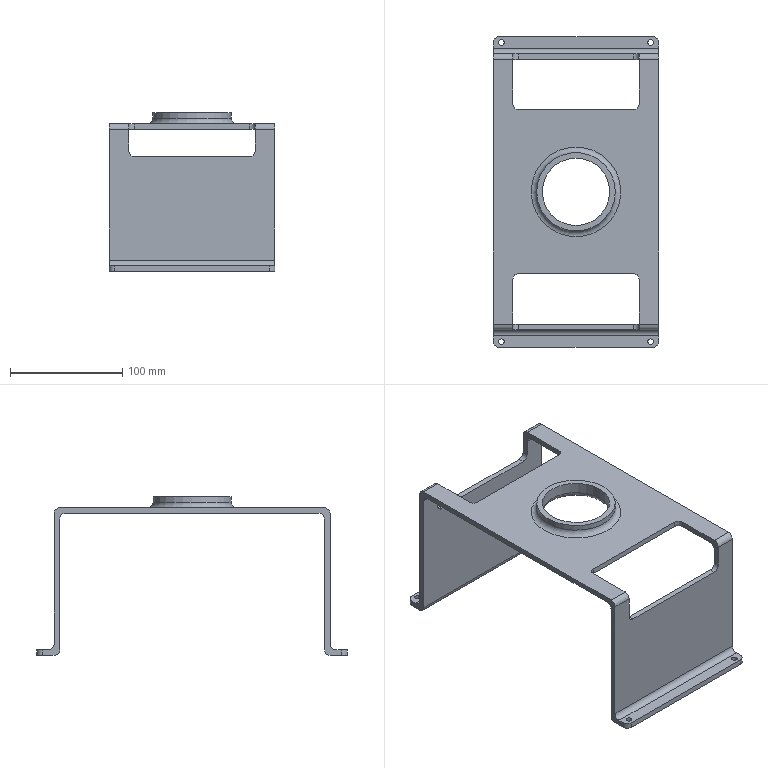Part | NX | features BREP 1 | 1 solid | 55 faces | box 147.796 x 276.466 x 141.5 mm | volume 303456 mm3 | cylinder 30 | plane 23 | torus 2 | commonest cylinder face diameters 10 x24 5 x4 60 x1 70 x1